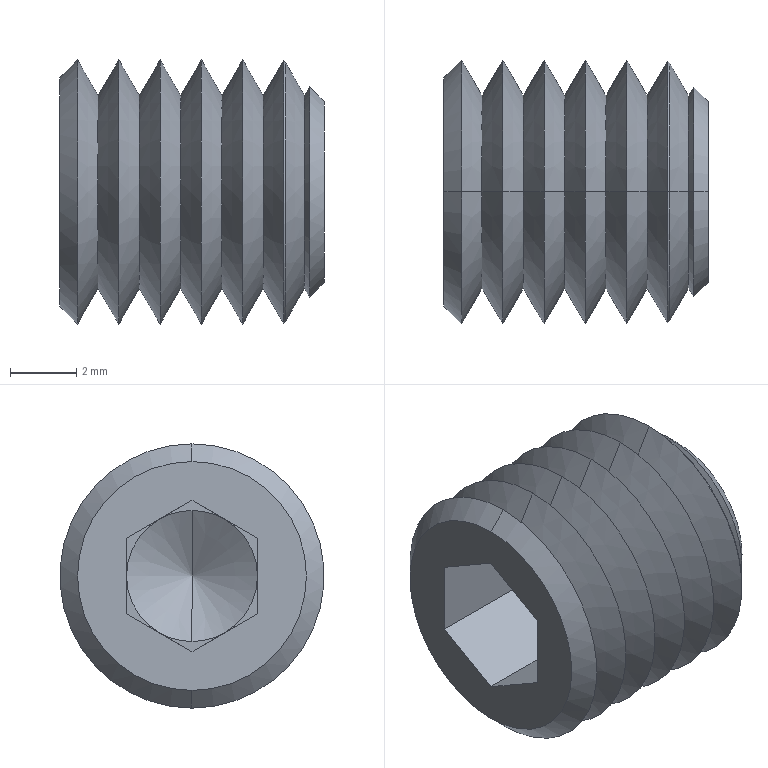Part | STEP file | GB/T 77 M8×8_M8×8 | 1 solid | 46 faces | box 8 x 8 x 8 mm | volume 254.883 mm3 | cone 32 | plane 14